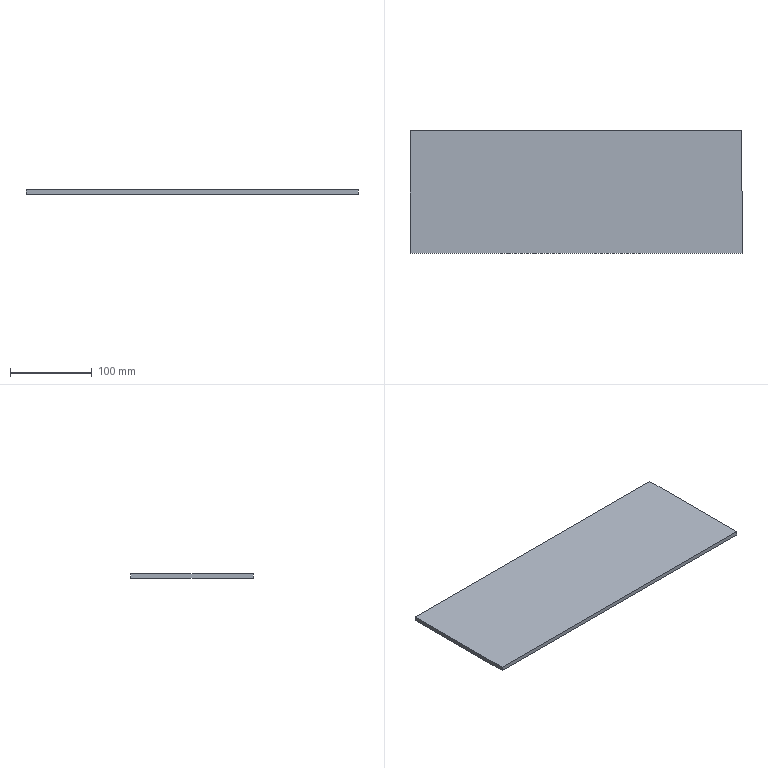Part | SolidWorks | features Extrusion 1 | 1 solid | 6 faces | box 405 x 150 x 5 mm | volume 303750 mm3 | plane 6
STEP:
#1=CARTESIAN_POINT('',(202.5,-75.,0.));
#2=VERTEX_POINT('',#1);
#3=CARTESIAN_POINT('',(202.5,75.,0.));
#4=VERTEX_POINT('',#3);
#5=CARTESIAN_POINT('',(202.5,75.,0.));
#6=DIRECTION('',(0.,1.,0.));
#7=VECTOR('',#6,1000.);
#8=LINE('',#5,#7);
#9=EDGE_CURVE('',#2,#4,#8,.T.);
#10=ORIENTED_EDGE('',*,*,#9,.T.);
#11=CARTESIAN_POINT('',(202.5,75.,5.));
#12=VERTEX_POINT('',#11);
#13=CARTESIAN_POINT('',(202.5,75.,5.));
#14=DIRECTION('',(0.,0.,-1.));
#15=VECTOR('',#14,1000.);
#16=LINE('',#13,#15);
#17=EDGE_CURVE('',#12,#4,#16,.T.);
#18=ORIENTED_EDGE('',*,*,#17,.F.);
#19=CARTESIAN_POINT('',(202.5,-75.,5.));
#20=VERTEX_POINT('',#19);
#21=CARTESIAN_POINT('',(202.5,75.,5.));
#22=DIRECTION('',(0.,1.,0.));
#23=VECTOR('',#22,1000.);
#24=LINE('',#21,#23);
#25=EDGE_CURVE('',#20,#12,#24,.T.);
#26=ORIENTED_EDGE('',*,*,#25,.F.);
#27=CARTESIAN_POINT('',(202.5,-75.,5.));
#28=DIRECTION('',(0.,0.,-1.));
#29=VECTOR('',#28,1000.);
#30=LINE('',#27,#29);
#31=EDGE_CURVE('',#20,#2,#30,.T.);
#32=ORIENTED_EDGE('',*,*,#31,.T.);
#33=EDGE_LOOP('',(#10,#18,#26,#32));
#34=FACE_OUTER_BOUND('',#33,.T.);
#35=CARTESIAN_POINT('',(202.5,75.,5.));
#36=DIRECTION('',(-1.,0.,0.));
#37=DIRECTION('',(0.,-1.,0.));
#38=AXIS2_PLACEMENT_3D('',#35,#36,#37);
#39=PLANE('',#38);
#40=ADVANCED_FACE('',(#34),#39,.F.);
#41=CARTESIAN_POINT('',(-202.5,75.,0.));
#42=VERTEX_POINT('',#41);
#43=CARTESIAN_POINT('',(-202.5,75.,0.));
#44=DIRECTION('',(-1.,0.,0.));
#45=VECTOR('',#44,1000.);
#46=LINE('',#43,#45);
#47=EDGE_CURVE('',#4,#42,#46,.T.);
#48=ORIENTED_EDGE('',*,*,#47,.T.);
#49=CARTESIAN_POINT('',(-202.5,75.,5.));
#50=VERTEX_POINT('',#49);
#51=CARTESIAN_POINT('',(-202.5,75.,5.));
#52=DIRECTION('',(0.,0.,-1.));
#53=VECTOR('',#52,1000.);
#54=LINE('',#51,#53);
#55=EDGE_CURVE('',#50,#42,#54,.T.);
#56=ORIENTED_EDGE('',*,*,#55,.F.);
#57=CARTESIAN_POINT('',(-202.5,75.,5.));
#58=DIRECTION('',(-1.,0.,0.));
#59=VECTOR('',#58,1000.);
#60=LINE('',#57,#59);
#61=EDGE_CURVE('',#12,#50,#60,.T.);
#62=ORIENTED_EDGE('',*,*,#61,.F.);
#63=ORIENTED_EDGE('',*,*,#17,.T.);
#64=EDGE_LOOP('',(#48,#56,#62,#63));
#65=FACE_OUTER_BOUND('',#64,.T.);
#66=CARTESIAN_POINT('',(-202.5,75.,5.));
#67=DIRECTION('',(0.,-1.,0.));
#68=DIRECTION('',(0.,0.,-1.));
#69=AXIS2_PLACEMENT_3D('',#66,#67,#68);
#70=PLANE('',#69);
#71=ADVANCED_FACE('',(#65),#70,.F.);
#72=CARTESIAN_POINT('',(-202.5,-75.,0.));
#73=VERTEX_POINT('',#72);
#74=CARTESIAN_POINT('',(-202.5,75.,0.));
#75=DIRECTION('',(0.,-1.,0.));
#76=VECTOR('',#75,1000.);
#77=LINE('',#74,#76);
#78=EDGE_CURVE('',#42,#73,#77,.T.);
#79=ORIENTED_EDGE('',*,*,#78,.T.);
#80=CARTESIAN_POINT('',(-202.5,-75.,5.));
#81=VERTEX_POINT('',#80);
#82=CARTESIAN_POINT('',(-202.5,-75.,5.));
#83=DIRECTION('',(0.,0.,-1.));
#84=VECTOR('',#83,1000.);
#85=LINE('',#82,#84);
#86=EDGE_CURVE('',#81,#73,#85,.T.);
#87=ORIENTED_EDGE('',*,*,#86,.F.);
#88=CARTESIAN_POINT('',(-202.5,75.,5.));
#89=DIRECTION('',(0.,-1.,0.));
#90=VECTOR('',#89,1000.);
#91=LINE('',#88,#90);
#92=EDGE_CURVE('',#50,#81,#91,.T.);
#93=ORIENTED_EDGE('',*,*,#92,.F.);
#94=ORIENTED_EDGE('',*,*,#55,.T.);
#95=EDGE_LOOP('',(#79,#87,#93,#94));
#96=FACE_OUTER_BOUND('',#95,.T.);
#97=CARTESIAN_POINT('',(-202.5,75.,5.));
#98=DIRECTION('',(1.,0.,0.));
#99=DIRECTION('',(0.,0.,-1.));
#100=AXIS2_PLACEMENT_3D('',#97,#98,#99);
#101=PLANE('',#100);
#102=ADVANCED_FACE('',(#96),#101,.F.);
#103=CARTESIAN_POINT('',(-202.5,-75.,0.));
#104=DIRECTION('',(1.,0.,0.));
#105=VECTOR('',#104,1000.);
#106=LINE('',#103,#105);
#107=EDGE_CURVE('',#73,#2,#106,.T.);
#108=ORIENTED_EDGE('',*,*,#107,.T.);
#109=ORIENTED_EDGE('',*,*,#31,.F.);
#110=CARTESIAN_POINT('',(-202.5,-75.,5.));
#111=DIRECTION('',(1.,0.,0.));
#112=VECTOR('',#111,1000.);
#113=LINE('',#110,#112);
#114=EDGE_CURVE('',#81,#20,#113,.T.);
#115=ORIENTED_EDGE('',*,*,#114,.F.);
#116=ORIENTED_EDGE('',*,*,#86,.T.);
#117=EDGE_LOOP('',(#108,#109,#115,#116));
#118=FACE_OUTER_BOUND('',#117,.T.);
#119=CARTESIAN_POINT('',(-202.5,-75.,5.));
#120=DIRECTION('',(0.,1.,0.));
#121=DIRECTION('',(0.,0.,1.));
#122=AXIS2_PLACEMENT_3D('',#119,#120,#121);
#123=PLANE('',#122);
#124=ADVANCED_FACE('',(#118),#123,.F.);
#125=ORIENTED_EDGE('',*,*,#25,.T.);
#126=ORIENTED_EDGE('',*,*,#61,.T.);
#127=ORIENTED_EDGE('',*,*,#92,.T.);
#128=ORIENTED_EDGE('',*,*,#114,.T.);
#129=EDGE_LOOP('',(#125,#126,#127,#128));
#130=FACE_OUTER_BOUND('',#129,.T.);
#131=CARTESIAN_POINT('',(0.,0.,5.));
#132=DIRECTION('',(0.,0.,1.));
#133=DIRECTION('',(1.,0.,0.));
#134=AXIS2_PLACEMENT_3D('',#131,#132,#133);
#135=PLANE('',#134);
#136=ADVANCED_FACE('',(#130),#135,.T.);
#137=ORIENTED_EDGE('',*,*,#9,.F.);
#138=ORIENTED_EDGE('',*,*,#107,.F.);
#139=ORIENTED_EDGE('',*,*,#78,.F.);
#140=ORIENTED_EDGE('',*,*,#47,.F.);
#141=EDGE_LOOP('',(#137,#138,#139,#140));
#142=FACE_OUTER_BOUND('',#141,.T.);
#143=CARTESIAN_POINT('',(0.,0.,0.));
#144=DIRECTION('',(0.,0.,1.));
#145=DIRECTION('',(1.,0.,0.));
#146=AXIS2_PLACEMENT_3D('',#143,#144,#145);
#147=PLANE('',#146);
#148=ADVANCED_FACE('',(#142),#147,.F.);
#149=CLOSED_SHELL('',(#40,#71,#102,#124,#136,#148));
#150=MANIFOLD_SOLID_BREP('',#149);
#151=CARTESIAN_POINT('',(0.,0.,0.));
#152=DIRECTION('',(0.,0.,1.));
#153=DIRECTION('',(1.,0.,0.));
#154=AXIS2_PLACEMENT_3D('',#151,#152,#153);
#155=(LENGTH_UNIT()NAMED_UNIT(*)SI_UNIT(.MILLI.,.METRE.));
#156=UNCERTAINTY_MEASURE_WITH_UNIT(LENGTH_MEASURE(0.00001),#155,'','');
#157=(NAMED_UNIT(*)PLANE_ANGLE_UNIT()SI_UNIT($,.RADIAN.));
#158=(NAMED_UNIT(*)SI_UNIT($,.STERADIAN.)SOLID_ANGLE_UNIT());
#159=(GEOMETRIC_REPRESENTATION_CONTEXT(3)GLOBAL_UNCERTAINTY_ASSIGNED_CONTEXT((#156))GLOBAL_UNIT_ASSIGNED_CONTEXT((#155,#157,#158))REPRESENTATION_CONTEXT('',''));
#160=ADVANCED_BREP_SHAPE_REPRESENTATION('',(#150,#154),#159);